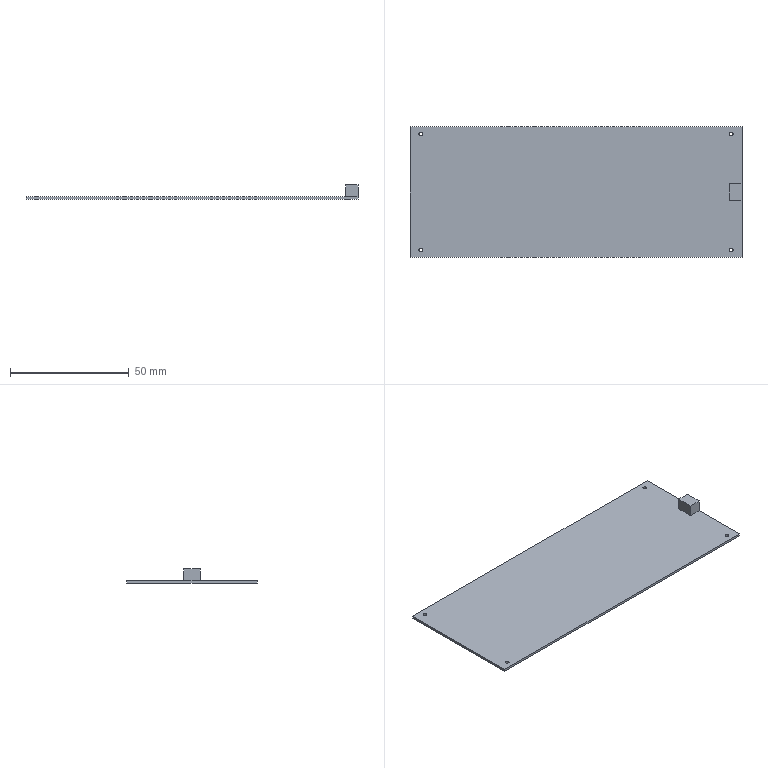Part | SolidWorks | features Extrusion 1, ICE 1 | 1 solid | 18 faces | box 140 x 55 x 6 mm | volume 7876 mm3 | plane 10 | cylinder 8 | commonest cylinder face diameters 1.5 x8
STEP:
#1=CARTESIAN_POINT('',(64.75,-24.5,1.));
#2=VERTEX_POINT('',#1);
#3=CARTESIAN_POINT('',(66.25,-24.5,1.));
#4=VERTEX_POINT('',#3);
#5=CARTESIAN_POINT('',(65.5,-24.5,1.));
#6=DIRECTION('',(0.,0.,1.));
#7=DIRECTION('',(1.,0.,0.));
#8=AXIS2_PLACEMENT_3D('',#5,#6,#7);
#9=CIRCLE('',#8,0.75);
#10=EDGE_CURVE('',#2,#4,#9,.T.);
#11=ORIENTED_EDGE('',*,*,#10,.T.);
#12=CARTESIAN_POINT('',(66.25,-24.5,0.));
#13=VERTEX_POINT('',#12);
#14=CARTESIAN_POINT('',(66.25,-24.5,1.));
#15=DIRECTION('',(0.,0.,-1.));
#16=VECTOR('',#15,1000.);
#17=LINE('',#14,#16);
#18=EDGE_CURVE('',#4,#13,#17,.T.);
#19=ORIENTED_EDGE('',*,*,#18,.T.);
#20=CARTESIAN_POINT('',(64.75,-24.5,0.));
#21=VERTEX_POINT('',#20);
#22=CARTESIAN_POINT('',(65.5,-24.5,0.));
#23=DIRECTION('',(0.,0.,1.));
#24=DIRECTION('',(1.,0.,0.));
#25=AXIS2_PLACEMENT_3D('',#22,#23,#24);
#26=CIRCLE('',#25,0.75);
#27=EDGE_CURVE('',#21,#13,#26,.T.);
#28=ORIENTED_EDGE('',*,*,#27,.F.);
#29=CARTESIAN_POINT('',(64.75,-24.5,1.));
#30=DIRECTION('',(0.,0.,-1.));
#31=VECTOR('',#30,1000.);
#32=LINE('',#29,#31);
#33=EDGE_CURVE('',#2,#21,#32,.T.);
#34=ORIENTED_EDGE('',*,*,#33,.F.);
#35=EDGE_LOOP('',(#11,#19,#28,#34));
#36=FACE_OUTER_BOUND('',#35,.T.);
#37=CARTESIAN_POINT('',(65.5,-24.5,1.));
#38=DIRECTION('',(0.,0.,-1.));
#39=DIRECTION('',(-1.,0.,0.));
#40=AXIS2_PLACEMENT_3D('',#37,#38,#39);
#41=CYLINDRICAL_SURFACE('',#40,0.75);
#42=ADVANCED_FACE('',(#36),#41,.F.);
#43=CARTESIAN_POINT('',(64.75,24.5,1.));
#44=VERTEX_POINT('',#43);
#45=CARTESIAN_POINT('',(66.25,24.5,1.));
#46=VERTEX_POINT('',#45);
#47=CARTESIAN_POINT('',(65.5,24.5,1.));
#48=DIRECTION('',(0.,0.,1.));
#49=DIRECTION('',(1.,0.,0.));
#50=AXIS2_PLACEMENT_3D('',#47,#48,#49);
#51=CIRCLE('',#50,0.75);
#52=EDGE_CURVE('',#44,#46,#51,.T.);
#53=ORIENTED_EDGE('',*,*,#52,.T.);
#54=CARTESIAN_POINT('',(66.25,24.5,0.));
#55=VERTEX_POINT('',#54);
#56=CARTESIAN_POINT('',(66.25,24.5,1.));
#57=DIRECTION('',(0.,0.,-1.));
#58=VECTOR('',#57,1000.);
#59=LINE('',#56,#58);
#60=EDGE_CURVE('',#46,#55,#59,.T.);
#61=ORIENTED_EDGE('',*,*,#60,.T.);
#62=CARTESIAN_POINT('',(64.75,24.5,0.));
#63=VERTEX_POINT('',#62);
#64=CARTESIAN_POINT('',(65.5,24.5,0.));
#65=DIRECTION('',(0.,0.,1.));
#66=DIRECTION('',(1.,0.,0.));
#67=AXIS2_PLACEMENT_3D('',#64,#65,#66);
#68=CIRCLE('',#67,0.75);
#69=EDGE_CURVE('',#63,#55,#68,.T.);
#70=ORIENTED_EDGE('',*,*,#69,.F.);
#71=CARTESIAN_POINT('',(64.75,24.5,1.));
#72=DIRECTION('',(0.,0.,-1.));
#73=VECTOR('',#72,1000.);
#74=LINE('',#71,#73);
#75=EDGE_CURVE('',#44,#63,#74,.T.);
#76=ORIENTED_EDGE('',*,*,#75,.F.);
#77=EDGE_LOOP('',(#53,#61,#70,#76));
#78=FACE_OUTER_BOUND('',#77,.T.);
#79=CARTESIAN_POINT('',(65.5,24.5,1.));
#80=DIRECTION('',(0.,0.,-1.));
#81=DIRECTION('',(-1.,0.,0.));
#82=AXIS2_PLACEMENT_3D('',#79,#80,#81);
#83=CYLINDRICAL_SURFACE('',#82,0.75);
#84=ADVANCED_FACE('',(#78),#83,.F.);
#85=CARTESIAN_POINT('',(-66.25,24.5,1.));
#86=VERTEX_POINT('',#85);
#87=CARTESIAN_POINT('',(-64.75,24.5,1.));
#88=VERTEX_POINT('',#87);
#89=CARTESIAN_POINT('',(-65.5,24.5,1.));
#90=DIRECTION('',(0.,0.,1.));
#91=DIRECTION('',(1.,0.,0.));
#92=AXIS2_PLACEMENT_3D('',#89,#90,#91);
#93=CIRCLE('',#92,0.75);
#94=EDGE_CURVE('',#86,#88,#93,.T.);
#95=ORIENTED_EDGE('',*,*,#94,.T.);
#96=CARTESIAN_POINT('',(-64.75,24.5,0.));
#97=VERTEX_POINT('',#96);
#98=CARTESIAN_POINT('',(-64.75,24.5,1.));
#99=DIRECTION('',(0.,0.,-1.));
#100=VECTOR('',#99,1000.);
#101=LINE('',#98,#100);
#102=EDGE_CURVE('',#88,#97,#101,.T.);
#103=ORIENTED_EDGE('',*,*,#102,.T.);
#104=CARTESIAN_POINT('',(-66.25,24.5,0.));
#105=VERTEX_POINT('',#104);
#106=CARTESIAN_POINT('',(-65.5,24.5,0.));
#107=DIRECTION('',(0.,0.,1.));
#108=DIRECTION('',(1.,0.,0.));
#109=AXIS2_PLACEMENT_3D('',#106,#107,#108);
#110=CIRCLE('',#109,0.75);
#111=EDGE_CURVE('',#105,#97,#110,.T.);
#112=ORIENTED_EDGE('',*,*,#111,.F.);
#113=CARTESIAN_POINT('',(-66.25,24.5,1.));
#114=DIRECTION('',(0.,0.,-1.));
#115=VECTOR('',#114,1000.);
#116=LINE('',#113,#115);
#117=EDGE_CURVE('',#86,#105,#116,.T.);
#118=ORIENTED_EDGE('',*,*,#117,.F.);
#119=EDGE_LOOP('',(#95,#103,#112,#118));
#120=FACE_OUTER_BOUND('',#119,.T.);
#121=CARTESIAN_POINT('',(-65.5,24.5,1.));
#122=DIRECTION('',(0.,0.,-1.));
#123=DIRECTION('',(-1.,0.,0.));
#124=AXIS2_PLACEMENT_3D('',#121,#122,#123);
#125=CYLINDRICAL_SURFACE('',#124,0.75);
#126=ADVANCED_FACE('',(#120),#125,.F.);
#127=CARTESIAN_POINT('',(-66.25,-24.5,1.));
#128=VERTEX_POINT('',#127);
#129=CARTESIAN_POINT('',(-64.75,-24.5,1.));
#130=VERTEX_POINT('',#129);
#131=CARTESIAN_POINT('',(-65.5,-24.5,1.));
#132=DIRECTION('',(0.,0.,1.));
#133=DIRECTION('',(1.,0.,0.));
#134=AXIS2_PLACEMENT_3D('',#131,#132,#133);
#135=CIRCLE('',#134,0.75);
#136=EDGE_CURVE('',#128,#130,#135,.T.);
#137=ORIENTED_EDGE('',*,*,#136,.T.);
#138=CARTESIAN_POINT('',(-64.75,-24.5,0.));
#139=VERTEX_POINT('',#138);
#140=CARTESIAN_POINT('',(-64.75,-24.5,1.));
#141=DIRECTION('',(0.,0.,-1.));
#142=VECTOR('',#141,1000.);
#143=LINE('',#140,#142);
#144=EDGE_CURVE('',#130,#139,#143,.T.);
#145=ORIENTED_EDGE('',*,*,#144,.T.);
#146=CARTESIAN_POINT('',(-66.25,-24.5,0.));
#147=VERTEX_POINT('',#146);
#148=CARTESIAN_POINT('',(-65.5,-24.5,0.));
#149=DIRECTION('',(0.,0.,1.));
#150=DIRECTION('',(1.,0.,0.));
#151=AXIS2_PLACEMENT_3D('',#148,#149,#150);
#152=CIRCLE('',#151,0.75);
#153=EDGE_CURVE('',#147,#139,#152,.T.);
#154=ORIENTED_EDGE('',*,*,#153,.F.);
#155=CARTESIAN_POINT('',(-66.25,-24.5,1.));
#156=DIRECTION('',(0.,0.,-1.));
#157=VECTOR('',#156,1000.);
#158=LINE('',#155,#157);
#159=EDGE_CURVE('',#128,#147,#158,.T.);
#160=ORIENTED_EDGE('',*,*,#159,.F.);
#161=EDGE_LOOP('',(#137,#145,#154,#160));
#162=FACE_OUTER_BOUND('',#161,.T.);
#163=CARTESIAN_POINT('',(-65.5,-24.5,1.));
#164=DIRECTION('',(0.,0.,-1.));
#165=DIRECTION('',(-1.,0.,0.));
#166=AXIS2_PLACEMENT_3D('',#163,#164,#165);
#167=CYLINDRICAL_SURFACE('',#166,0.75);
#168=ADVANCED_FACE('',(#162),#167,.F.);
#169=CARTESIAN_POINT('',(64.791,-3.512,1.));
#170=VERTEX_POINT('',#169);
#171=CARTESIAN_POINT('',(70.,-3.512,1.));
#172=VERTEX_POINT('',#171);
#173=CARTESIAN_POINT('',(64.791,-3.512,1.));
#174=DIRECTION('',(1.,0.,0.));
#175=VECTOR('',#174,1000.);
#176=LINE('',#173,#175);
#177=EDGE_CURVE('',#170,#172,#176,.T.);
#178=ORIENTED_EDGE('',*,*,#177,.F.);
#179=CARTESIAN_POINT('',(64.791,3.512,1.));
#180=VERTEX_POINT('',#179);
#181=CARTESIAN_POINT('',(64.791,3.512,1.));
#182=DIRECTION('',(0.,-1.,0.));
#183=VECTOR('',#182,1000.);
#184=LINE('',#181,#183);
#185=EDGE_CURVE('',#180,#170,#184,.T.);
#186=ORIENTED_EDGE('',*,*,#185,.F.);
#187=CARTESIAN_POINT('',(70.,3.512,1.));
#188=VERTEX_POINT('',#187);
#189=CARTESIAN_POINT('',(64.791,3.512,1.));
#190=DIRECTION('',(-1.,0.,0.));
#191=VECTOR('',#190,1000.);
#192=LINE('',#189,#191);
#193=EDGE_CURVE('',#188,#180,#192,.T.);
#194=ORIENTED_EDGE('',*,*,#193,.F.);
#195=CARTESIAN_POINT('',(70.,27.5,1.));
#196=VERTEX_POINT('',#195);
#197=CARTESIAN_POINT('',(70.,27.5,1.));
#198=DIRECTION('',(0.,1.,0.));
#199=VECTOR('',#198,1000.);
#200=LINE('',#197,#199);
#201=EDGE_CURVE('',#188,#196,#200,.T.);
#202=ORIENTED_EDGE('',*,*,#201,.T.);
#203=CARTESIAN_POINT('',(-70.,27.5,1.));
#204=VERTEX_POINT('',#203);
#205=CARTESIAN_POINT('',(-70.,27.5,1.));
#206=DIRECTION('',(-1.,0.,0.));
#207=VECTOR('',#206,1000.);
#208=LINE('',#205,#207);
#209=EDGE_CURVE('',#196,#204,#208,.T.);
#210=ORIENTED_EDGE('',*,*,#209,.T.);
#211=CARTESIAN_POINT('',(-70.,-27.5,1.));
#212=VERTEX_POINT('',#211);
#213=CARTESIAN_POINT('',(-70.,27.5,1.));
#214=DIRECTION('',(0.,-1.,0.));
#215=VECTOR('',#214,1000.);
#216=LINE('',#213,#215);
#217=EDGE_CURVE('',#204,#212,#216,.T.);
#218=ORIENTED_EDGE('',*,*,#217,.T.);
#219=CARTESIAN_POINT('',(70.,-27.5,1.));
#220=VERTEX_POINT('',#219);
#221=CARTESIAN_POINT('',(-70.,-27.5,1.));
#222=DIRECTION('',(1.,0.,0.));
#223=VECTOR('',#222,1000.);
#224=LINE('',#221,#223);
#225=EDGE_CURVE('',#212,#220,#224,.T.);
#226=ORIENTED_EDGE('',*,*,#225,.T.);
#227=CARTESIAN_POINT('',(70.,27.5,1.));
#228=DIRECTION('',(0.,1.,0.));
#229=VECTOR('',#228,1000.);
#230=LINE('',#227,#229);
#231=EDGE_CURVE('',#220,#172,#230,.T.);
#232=ORIENTED_EDGE('',*,*,#231,.T.);
#233=EDGE_LOOP('',(#178,#186,#194,#202,#210,#218,#226,#232));
#234=FACE_OUTER_BOUND('',#233,.T.);
#235=ORIENTED_EDGE('',*,*,#52,.F.);
#236=CARTESIAN_POINT('',(65.5,24.5,1.));
#237=DIRECTION('',(0.,0.,1.));
#238=DIRECTION('',(1.,0.,0.));
#239=AXIS2_PLACEMENT_3D('',#236,#237,#238);
#240=CIRCLE('',#239,0.75);
#241=EDGE_CURVE('',#46,#44,#240,.T.);
#242=ORIENTED_EDGE('',*,*,#241,.F.);
#243=EDGE_LOOP('',(#235,#242));
#244=FACE_BOUND('',#243,.T.);
#245=ORIENTED_EDGE('',*,*,#136,.F.);
#246=CARTESIAN_POINT('',(-65.5,-24.5,1.));
#247=DIRECTION('',(0.,0.,1.));
#248=DIRECTION('',(1.,0.,0.));
#249=AXIS2_PLACEMENT_3D('',#246,#247,#248);
#250=CIRCLE('',#249,0.75);
#251=EDGE_CURVE('',#130,#128,#250,.T.);
#252=ORIENTED_EDGE('',*,*,#251,.F.);
#253=EDGE_LOOP('',(#245,#252));
#254=FACE_BOUND('',#253,.T.);
#255=ORIENTED_EDGE('',*,*,#94,.F.);
#256=CARTESIAN_POINT('',(-65.5,24.5,1.));
#257=DIRECTION('',(0.,0.,1.));
#258=DIRECTION('',(1.,0.,0.));
#259=AXIS2_PLACEMENT_3D('',#256,#257,#258);
#260=CIRCLE('',#259,0.75);
#261=EDGE_CURVE('',#88,#86,#260,.T.);
#262=ORIENTED_EDGE('',*,*,#261,.F.);
#263=EDGE_LOOP('',(#255,#262));
#264=FACE_BOUND('',#263,.T.);
#265=ORIENTED_EDGE('',*,*,#10,.F.);
#266=CARTESIAN_POINT('',(65.5,-24.5,1.));
#267=DIRECTION('',(0.,0.,1.));
#268=DIRECTION('',(1.,0.,0.));
#269=AXIS2_PLACEMENT_3D('',#266,#267,#268);
#270=CIRCLE('',#269,0.75);
#271=EDGE_CURVE('',#4,#2,#270,.T.);
#272=ORIENTED_EDGE('',*,*,#271,.F.);
#273=EDGE_LOOP('',(#265,#272));
#274=FACE_BOUND('',#273,.T.);
#275=CARTESIAN_POINT('',(0.,0.,1.));
#276=DIRECTION('',(0.,0.,1.));
#277=DIRECTION('',(1.,0.,0.));
#278=AXIS2_PLACEMENT_3D('',#275,#276,#277);
#279=PLANE('',#278);
#280=ADVANCED_FACE('',(#234,#244,#254,#264,#274),#279,.T.);
#281=CARTESIAN_POINT('',(70.,-27.5,0.));
#282=VERTEX_POINT('',#281);
#283=CARTESIAN_POINT('',(70.,27.5,0.));
#284=VERTEX_POINT('',#283);
#285=CARTESIAN_POINT('',(70.,27.5,0.));
#286=DIRECTION('',(0.,1.,0.));
#287=VECTOR('',#286,1000.);
#288=LINE('',#285,#287);
#289=EDGE_CURVE('',#282,#284,#288,.T.);
#290=ORIENTED_EDGE('',*,*,#289,.F.);
#291=CARTESIAN_POINT('',(-70.,-27.5,0.));
#292=VERTEX_POINT('',#291);
#293=CARTESIAN_POINT('',(-70.,-27.5,0.));
#294=DIRECTION('',(1.,0.,0.));
#295=VECTOR('',#294,1000.);
#296=LINE('',#293,#295);
#297=EDGE_CURVE('',#292,#282,#296,.T.);
#298=ORIENTED_EDGE('',*,*,#297,.F.);
#299=CARTESIAN_POINT('',(-70.,27.5,0.));
#300=VERTEX_POINT('',#299);
#301=CARTESIAN_POINT('',(-70.,27.5,0.));
#302=DIRECTION('',(0.,-1.,0.));
#303=VECTOR('',#302,1000.);
#304=LINE('',#301,#303);
#305=EDGE_CURVE('',#300,#292,#304,.T.);
#306=ORIENTED_EDGE('',*,*,#305,.F.);
#307=CARTESIAN_POINT('',(-70.,27.5,0.));
#308=DIRECTION('',(-1.,0.,0.));
#309=VECTOR('',#308,1000.);
#310=LINE('',#307,#309);
#311=EDGE_CURVE('',#284,#300,#310,.T.);
#312=ORIENTED_EDGE('',*,*,#311,.F.);
#313=EDGE_LOOP('',(#290,#298,#306,#312));
#314=FACE_OUTER_BOUND('',#313,.T.);
#315=ORIENTED_EDGE('',*,*,#153,.T.);
#316=CARTESIAN_POINT('',(-65.5,-24.5,0.));
#317=DIRECTION('',(0.,0.,1.));
#318=DIRECTION('',(1.,0.,0.));
#319=AXIS2_PLACEMENT_3D('',#316,#317,#318);
#320=CIRCLE('',#319,0.75);
#321=EDGE_CURVE('',#139,#147,#320,.T.);
#322=ORIENTED_EDGE('',*,*,#321,.T.);
#323=EDGE_LOOP('',(#315,#322));
#324=FACE_BOUND('',#323,.T.);
#325=ORIENTED_EDGE('',*,*,#111,.T.);
#326=CARTESIAN_POINT('',(-65.5,24.5,0.));
#327=DIRECTION('',(0.,0.,1.));
#328=DIRECTION('',(1.,0.,0.));
#329=AXIS2_PLACEMENT_3D('',#326,#327,#328);
#330=CIRCLE('',#329,0.75);
#331=EDGE_CURVE('',#97,#105,#330,.T.);
#332=ORIENTED_EDGE('',*,*,#331,.T.);
#333=EDGE_LOOP('',(#325,#332));
#334=FACE_BOUND('',#333,.T.);
#335=ORIENTED_EDGE('',*,*,#69,.T.);
#336=CARTESIAN_POINT('',(65.5,24.5,0.));
#337=DIRECTION('',(0.,0.,1.));
#338=DIRECTION('',(1.,0.,0.));
#339=AXIS2_PLACEMENT_3D('',#336,#337,#338);
#340=CIRCLE('',#339,0.75);
#341=EDGE_CURVE('',#55,#63,#340,.T.);
#342=ORIENTED_EDGE('',*,*,#341,.T.);
#343=EDGE_LOOP('',(#335,#342));
#344=FACE_BOUND('',#343,.T.);
#345=ORIENTED_EDGE('',*,*,#27,.T.);
#346=CARTESIAN_POINT('',(65.5,-24.5,0.));
#347=DIRECTION('',(0.,0.,1.));
#348=DIRECTION('',(1.,0.,0.));
#349=AXIS2_PLACEMENT_3D('',#346,#347,#348);
#350=CIRCLE('',#349,0.75);
#351=EDGE_CURVE('',#13,#21,#350,.T.);
#352=ORIENTED_EDGE('',*,*,#351,.T.);
#353=EDGE_LOOP('',(#345,#352));
#354=FACE_BOUND('',#353,.T.);
#355=CARTESIAN_POINT('',(0.,0.,0.));
#356=DIRECTION('',(0.,0.,1.));
#357=DIRECTION('',(1.,0.,0.));
#358=AXIS2_PLACEMENT_3D('',#355,#356,#357);
#359=PLANE('',#358);
#360=ADVANCED_FACE('',(#314,#324,#334,#344,#354),#359,.F.);
#361=ORIENTED_EDGE('',*,*,#289,.T.);
#362=CARTESIAN_POINT('',(70.,27.5,1.));
#363=DIRECTION('',(0.,0.,-1.));
#364=VECTOR('',#363,1000.);
#365=LINE('',#362,#364);
#366=EDGE_CURVE('',#196,#284,#365,.T.);
#367=ORIENTED_EDGE('',*,*,#366,.F.);
#368=ORIENTED_EDGE('',*,*,#201,.F.);
#369=CARTESIAN_POINT('',(70.,3.512,6.));
#370=VERTEX_POINT('',#369);
#371=CARTESIAN_POINT('',(70.,3.512,6.));
#372=DIRECTION('',(0.,0.,-1.));
#373=VECTOR('',#372,1000.);
#374=LINE('',#371,#373);
#375=EDGE_CURVE('',#370,#188,#374,.T.);
#376=ORIENTED_EDGE('',*,*,#375,.F.);
#377=CARTESIAN_POINT('',(70.,-3.512,6.));
#378=VERTEX_POINT('',#377);
#379=CARTESIAN_POINT('',(70.,3.512,6.));
#380=DIRECTION('',(0.,1.,0.));
#381=VECTOR('',#380,1000.);
#382=LINE('',#379,#381);
#383=EDGE_CURVE('',#378,#370,#382,.T.);
#384=ORIENTED_EDGE('',*,*,#383,.F.);
#385=CARTESIAN_POINT('',(70.,-3.512,6.));
#386=DIRECTION('',(0.,0.,-1.));
#387=VECTOR('',#386,1000.);
#388=LINE('',#385,#387);
#389=EDGE_CURVE('',#378,#172,#388,.T.);
#390=ORIENTED_EDGE('',*,*,#389,.T.);
#391=ORIENTED_EDGE('',*,*,#231,.F.);
#392=CARTESIAN_POINT('',(70.,-27.5,1.));
#393=DIRECTION('',(0.,0.,-1.));
#394=VECTOR('',#393,1000.);
#395=LINE('',#392,#394);
#396=EDGE_CURVE('',#220,#282,#395,.T.);
#397=ORIENTED_EDGE('',*,*,#396,.T.);
#398=EDGE_LOOP('',(#361,#367,#368,#376,#384,#390,#391,#397));
#399=FACE_OUTER_BOUND('',#398,.T.);
#400=CARTESIAN_POINT('',(70.,27.5,1.));
#401=DIRECTION('',(-1.,0.,0.));
#402=DIRECTION('',(0.,0.,1.));
#403=AXIS2_PLACEMENT_3D('',#400,#401,#402);
#404=PLANE('',#403);
#405=ADVANCED_FACE('',(#399),#404,.F.);
#406=ORIENTED_EDGE('',*,*,#311,.T.);
#407=CARTESIAN_POINT('',(-70.,27.5,1.));
#408=DIRECTION('',(0.,0.,-1.));
#409=VECTOR('',#408,1000.);
#410=LINE('',#407,#409);
#411=EDGE_CURVE('',#204,#300,#410,.T.);
#412=ORIENTED_EDGE('',*,*,#411,.F.);
#413=ORIENTED_EDGE('',*,*,#209,.F.);
#414=ORIENTED_EDGE('',*,*,#366,.T.);
#415=EDGE_LOOP('',(#406,#412,#413,#414));
#416=FACE_OUTER_BOUND('',#415,.T.);
#417=CARTESIAN_POINT('',(-70.,27.5,1.));
#418=DIRECTION('',(0.,-1.,0.));
#419=DIRECTION('',(1.,0.,0.));
#420=AXIS2_PLACEMENT_3D('',#417,#418,#419);
#421=PLANE('',#420);
#422=ADVANCED_FACE('',(#416),#421,.F.);
#423=ORIENTED_EDGE('',*,*,#305,.T.);
#424=CARTESIAN_POINT('',(-70.,-27.5,1.));
#425=DIRECTION('',(0.,0.,-1.));
#426=VECTOR('',#425,1000.);
#427=LINE('',#424,#426);
#428=EDGE_CURVE('',#212,#292,#427,.T.);
#429=ORIENTED_EDGE('',*,*,#428,.F.);
#430=ORIENTED_EDGE('',*,*,#217,.F.);
#431=ORIENTED_EDGE('',*,*,#411,.T.);
#432=EDGE_LOOP('',(#423,#429,#430,#431));
#433=FACE_OUTER_BOUND('',#432,.T.);
#434=CARTESIAN_POINT('',(-70.,27.5,1.));
#435=DIRECTION('',(1.,0.,0.));
#436=DIRECTION('',(0.,0.,-1.));
#437=AXIS2_PLACEMENT_3D('',#434,#435,#436);
#438=PLANE('',#437);
#439=ADVANCED_FACE('',(#433),#438,.F.);
#440=ORIENTED_EDGE('',*,*,#297,.T.);
#441=ORIENTED_EDGE('',*,*,#396,.F.);
#442=ORIENTED_EDGE('',*,*,#225,.F.);
#443=ORIENTED_EDGE('',*,*,#428,.T.);
#444=EDGE_LOOP('',(#440,#441,#442,#443));
#445=FACE_OUTER_BOUND('',#444,.T.);
#446=CARTESIAN_POINT('',(-70.,-27.5,1.));
#447=DIRECTION('',(0.,1.,0.));
#448=DIRECTION('',(0.,0.,1.));
#449=AXIS2_PLACEMENT_3D('',#446,#447,#448);
#450=PLANE('',#449);
#451=ADVANCED_FACE('',(#445),#450,.F.);
#452=ORIENTED_EDGE('',*,*,#144,.F.);
#453=ORIENTED_EDGE('',*,*,#251,.T.);
#454=ORIENTED_EDGE('',*,*,#159,.T.);
#455=ORIENTED_EDGE('',*,*,#321,.F.);
#456=EDGE_LOOP('',(#452,#453,#454,#455));
#457=FACE_OUTER_BOUND('',#456,.T.);
#458=CARTESIAN_POINT('',(-65.5,-24.5,1.));
#459=DIRECTION('',(0.,0.,-1.));
#460=DIRECTION('',(-1.,0.,0.));
#461=AXIS2_PLACEMENT_3D('',#458,#459,#460);
#462=CYLINDRICAL_SURFACE('',#461,0.75);
#463=ADVANCED_FACE('',(#457),#462,.F.);
#464=ORIENTED_EDGE('',*,*,#102,.F.);
#465=ORIENTED_EDGE('',*,*,#261,.T.);
#466=ORIENTED_EDGE('',*,*,#117,.T.);
#467=ORIENTED_EDGE('',*,*,#331,.F.);
#468=EDGE_LOOP('',(#464,#465,#466,#467));
#469=FACE_OUTER_BOUND('',#468,.T.);
#470=CARTESIAN_POINT('',(-65.5,24.5,1.));
#471=DIRECTION('',(0.,0.,-1.));
#472=DIRECTION('',(-1.,0.,0.));
#473=AXIS2_PLACEMENT_3D('',#470,#471,#472);
#474=CYLINDRICAL_SURFACE('',#473,0.75);
#475=ADVANCED_FACE('',(#469),#474,.F.);
#476=ORIENTED_EDGE('',*,*,#60,.F.);
#477=ORIENTED_EDGE('',*,*,#241,.T.);
#478=ORIENTED_EDGE('',*,*,#75,.T.);
#479=ORIENTED_EDGE('',*,*,#341,.F.);
#480=EDGE_LOOP('',(#476,#477,#478,#479));
#481=FACE_OUTER_BOUND('',#480,.T.);
#482=CARTESIAN_POINT('',(65.5,24.5,1.));
#483=DIRECTION('',(0.,0.,-1.));
#484=DIRECTION('',(-1.,0.,0.));
#485=AXIS2_PLACEMENT_3D('',#482,#483,#484);
#486=CYLINDRICAL_SURFACE('',#485,0.75);
#487=ADVANCED_FACE('',(#481),#486,.F.);
#488=ORIENTED_EDGE('',*,*,#18,.F.);
#489=ORIENTED_EDGE('',*,*,#271,.T.);
#490=ORIENTED_EDGE('',*,*,#33,.T.);
#491=ORIENTED_EDGE('',*,*,#351,.F.);
#492=EDGE_LOOP('',(#488,#489,#490,#491));
#493=FACE_OUTER_BOUND('',#492,.T.);
#494=CARTESIAN_POINT('',(65.5,-24.5,1.));
#495=DIRECTION('',(0.,0.,-1.));
#496=DIRECTION('',(-1.,0.,0.));
#497=AXIS2_PLACEMENT_3D('',#494,#495,#496);
#498=CYLINDRICAL_SURFACE('',#497,0.75);
#499=ADVANCED_FACE('',(#493),#498,.F.);
#500=ORIENTED_EDGE('',*,*,#193,.T.);
#501=CARTESIAN_POINT('',(64.791,3.512,6.));
#502=VERTEX_POINT('',#501);
#503=CARTESIAN_POINT('',(64.791,3.512,6.));
#504=DIRECTION('',(0.,0.,-1.));
#505=VECTOR('',#504,1000.);
#506=LINE('',#503,#505);
#507=EDGE_CURVE('',#502,#180,#506,.T.);
#508=ORIENTED_EDGE('',*,*,#507,.F.);
#509=CARTESIAN_POINT('',(64.791,3.512,6.));
#510=DIRECTION('',(-1.,0.,0.));
#511=VECTOR('',#510,1000.);
#512=LINE('',#509,#511);
#513=EDGE_CURVE('',#370,#502,#512,.T.);
#514=ORIENTED_EDGE('',*,*,#513,.F.);
#515=ORIENTED_EDGE('',*,*,#375,.T.);
#516=EDGE_LOOP('',(#500,#508,#514,#515));
#517=FACE_OUTER_BOUND('',#516,.T.);
#518=CARTESIAN_POINT('',(64.791,3.512,6.));
#519=DIRECTION('',(0.,-1.,0.));
#520=DIRECTION('',(0.,0.,-1.));
#521=AXIS2_PLACEMENT_3D('',#518,#519,#520);
#522=PLANE('',#521);
#523=ADVANCED_FACE('',(#517),#522,.F.);
#524=ORIENTED_EDGE('',*,*,#185,.T.);
#525=CARTESIAN_POINT('',(64.791,-3.512,6.));
#526=VERTEX_POINT('',#525);
#527=CARTESIAN_POINT('',(64.791,-3.512,6.));
#528=DIRECTION('',(0.,0.,-1.));
#529=VECTOR('',#528,1000.);
#530=LINE('',#527,#529);
#531=EDGE_CURVE('',#526,#170,#530,.T.);
#532=ORIENTED_EDGE('',*,*,#531,.F.);
#533=CARTESIAN_POINT('',(64.791,3.512,6.));
#534=DIRECTION('',(0.,-1.,0.));
#535=VECTOR('',#534,1000.);
#536=LINE('',#533,#535);
#537=EDGE_CURVE('',#502,#526,#536,.T.);
#538=ORIENTED_EDGE('',*,*,#537,.F.);
#539=ORIENTED_EDGE('',*,*,#507,.T.);
#540=EDGE_LOOP('',(#524,#532,#538,#539));
#541=FACE_OUTER_BOUND('',#540,.T.);
#542=CARTESIAN_POINT('',(64.791,3.512,6.));
#543=DIRECTION('',(1.,0.,0.));
#544=DIRECTION('',(0.,0.,-1.));
#545=AXIS2_PLACEMENT_3D('',#542,#543,#544);
#546=PLANE('',#545);
#547=ADVANCED_FACE('',(#541),#546,.F.);
#548=ORIENTED_EDGE('',*,*,#177,.T.);
#549=ORIENTED_EDGE('',*,*,#389,.F.);
#550=CARTESIAN_POINT('',(64.791,-3.512,6.));
#551=DIRECTION('',(1.,0.,0.));
#552=VECTOR('',#551,1000.);
#553=LINE('',#550,#552);
#554=EDGE_CURVE('',#526,#378,#553,.T.);
#555=ORIENTED_EDGE('',*,*,#554,.F.);
#556=ORIENTED_EDGE('',*,*,#531,.T.);
#557=EDGE_LOOP('',(#548,#549,#555,#556));
#558=FACE_OUTER_BOUND('',#557,.T.);
#559=CARTESIAN_POINT('',(64.791,-3.512,6.));
#560=DIRECTION('',(0.,1.,0.));
#561=DIRECTION('',(0.,0.,1.));
#562=AXIS2_PLACEMENT_3D('',#559,#560,#561);
#563=PLANE('',#562);
#564=ADVANCED_FACE('',(#558),#563,.F.);
#565=ORIENTED_EDGE('',*,*,#383,.T.);
#566=ORIENTED_EDGE('',*,*,#513,.T.);
#567=ORIENTED_EDGE('',*,*,#537,.T.);
#568=ORIENTED_EDGE('',*,*,#554,.T.);
#569=EDGE_LOOP('',(#565,#566,#567,#568));
#570=FACE_OUTER_BOUND('',#569,.T.);
#571=CARTESIAN_POINT('',(0.,0.,6.));
#572=DIRECTION('',(0.,0.,1.));
#573=DIRECTION('',(1.,0.,0.));
#574=AXIS2_PLACEMENT_3D('',#571,#572,#573);
#575=PLANE('',#574);
#576=ADVANCED_FACE('',(#570),#575,.T.);
#577=CLOSED_SHELL('',(#42,#84,#126,#168,#280,#360,#405,#422,#439,#451,#463,#475,#487,#499,#523,#547,#564,#576));
#578=MANIFOLD_SOLID_BREP('',#577);
#579=CARTESIAN_POINT('',(0.,0.,0.));
#580=DIRECTION('',(0.,0.,1.));
#581=DIRECTION('',(1.,0.,0.));
#582=AXIS2_PLACEMENT_3D('',#579,#580,#581);
#583=(LENGTH_UNIT()NAMED_UNIT(*)SI_UNIT(.MILLI.,.METRE.));
#584=UNCERTAINTY_MEASURE_WITH_UNIT(LENGTH_MEASURE(0.00001),#583,'','');
#585=(NAMED_UNIT(*)PLANE_ANGLE_UNIT()SI_UNIT($,.RADIAN.));
#586=(NAMED_UNIT(*)SI_UNIT($,.STERADIAN.)SOLID_ANGLE_UNIT());
#587=(GEOMETRIC_REPRESENTATION_CONTEXT(3)GLOBAL_UNCERTAINTY_ASSIGNED_CONTEXT((#584))GLOBAL_UNIT_ASSIGNED_CONTEXT((#583,#585,#586))REPRESENTATION_CONTEXT('',''));
#588=ADVANCED_BREP_SHAPE_REPRESENTATION('',(#578,#582),#587);